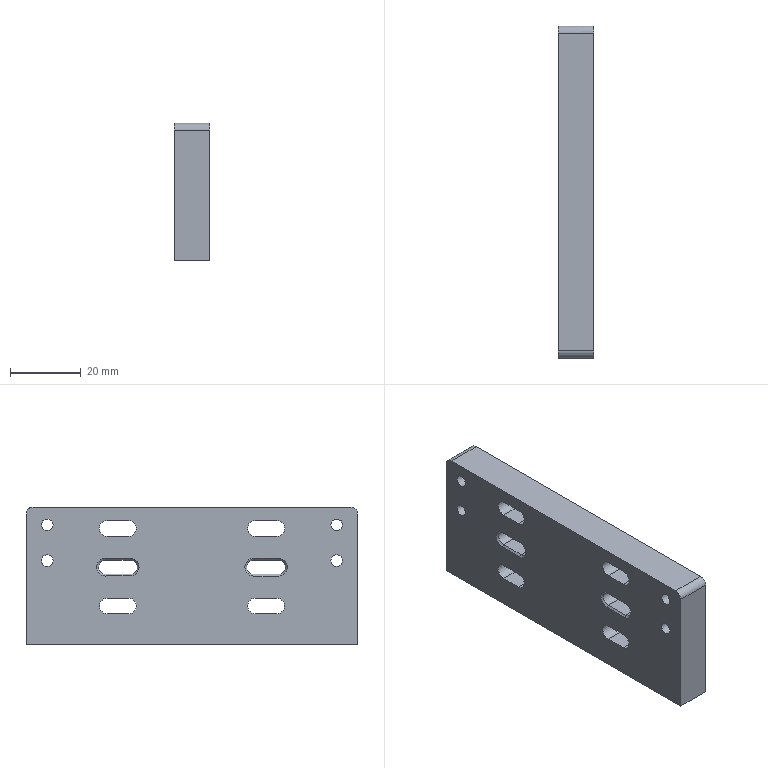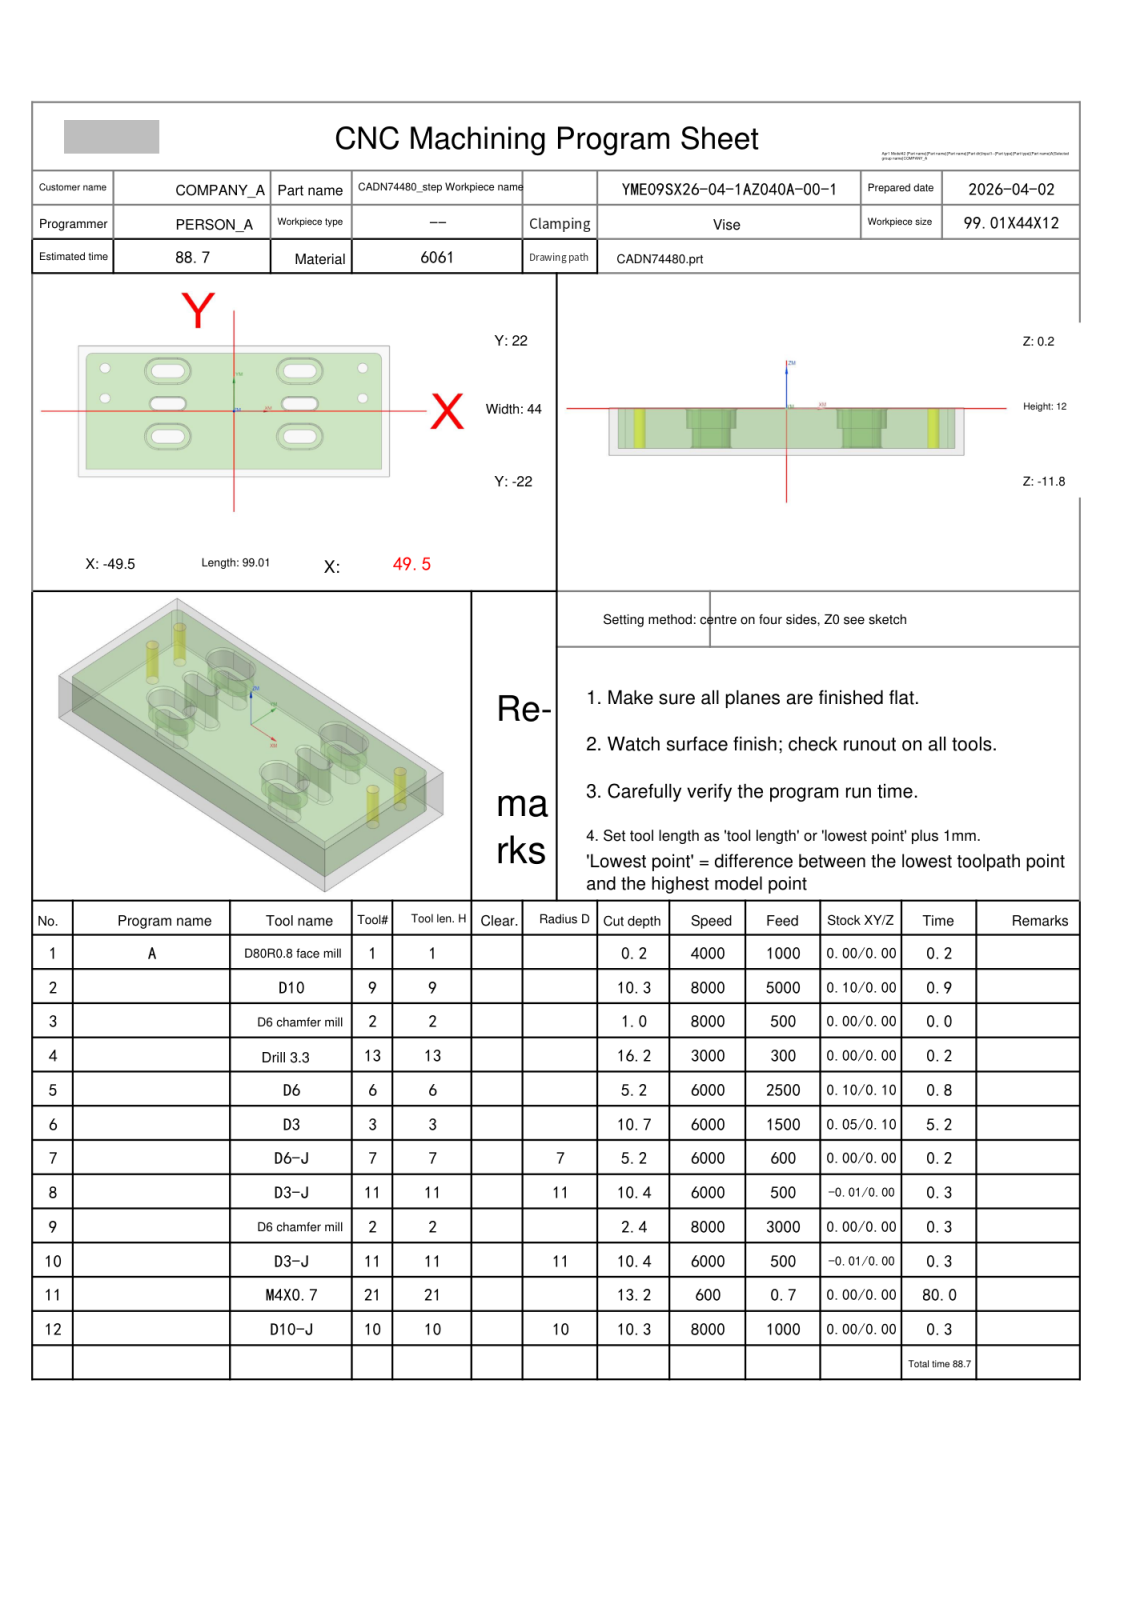NC program | NX | posted by the shop | part box 10.067 x 94 x 39 mm
Lines 1 to 937 of 4590:
%
O0001
(Machine time: 165.52 MIN)
(===Total Tool:10===)
(T1=D80R0.8 face mill D=80.  R=0.8  D-  H01 Z=0.    )
(T9=D10     D=10.  R=0.   D-  H09 Z=-10.1 )
(T2=D6 chamfer mill   D=6.   R=0.   D-  H02 Z=-2.2  )
(T13=Drill 3.3  D=3.3  DR_a=118 D-  H13 Z=-15.99)
(T6=D6      D=6.   R=0.   D-  H06 Z=-5.   )
(T3=D3      D=3.   R=0.   D-  H03 Z=-10.5 )
(T7=D6-J    D=6.   R=0.   D7  H07 Z=-5.   )
(T11=D3-J   D=3.   R=0.   D11 H11 Z=-10.2 )
(T21=M4X0.7 D=3.3  DR_a=180 D-  H21 Z=-13.  )
(T10=D10-J  D=10.  R=0.   D10 H10 Z=-10.1 )
G80 G90 G17 G49 G40
G91 G28 Z0
M01
N1 T01 M06
(D80R0.8 face mill  D=80. R=0.8 H=01 ce=0.00 di=0.00)
G00 G90 G54 X-92.004 Y0.0 M03 S4000
G43 H01 Z20.
M08
Z2.
G01 Z0.0 F1000.
X-87.004
X87.004
X92.004
Z2.
G00 Z20.
G91 G28 Z0.0
M05
M09
G91 G28 Z0.0
M01
N2 T09 M06
(D10  D=10. R=0. H=09 ce=0.10 di=0.00)
G00 G90 G54 X0.0 Y-24.6 M03 S8000
G43 H09 Z20.
M08
Z.5
G01 X-47.004 Z.38 F5000.
G02 X-52.104 Y-19.5 Z.359 I0.0 J5.1
G01 Y17.5 Z.265
G02 X-45.004 Y24.6 Z.236 I7.1 J0.0
G01 X45.004 Z.006
G02 X52.104 Y17.5 Z-.022 I0.0 J-7.1
G01 Y-19.5 Z-.117
G02 X47.004 Y-24.6 Z-.137 I-5.1 J0.0
G01 X-47.004 Z-.377
G02 X-52.104 Y-19.5 Z-.398 I0.0 J5.1
G01 Y17.5 Z-.492
G02 X-45.004 Y24.6 Z-.521 I7.1 J0.0
G01 X45.004 Z-.751
G02 X52.104 Y17.5 Z-.779 I0.0 J-7.1
G01 Y-19.5 Z-.874
G02 X47.004 Y-24.6 Z-.894 I-5.1 J0.0
G01 X-47.004 Z-1.134
G02 X-52.104 Y-19.5 Z-1.155 I0.0 J5.1
G01 Y17.5 Z-1.249
G02 X-45.004 Y24.6 Z-1.278 I7.1 J0.0
G01 X45.004 Z-1.508
G02 X52.104 Y17.5 Z-1.536 I0.0 J-7.1
G01 Y-19.5 Z-1.631
G02 X47.004 Y-24.6 Z-1.651 I-5.1 J0.0
G01 X-47.004 Z-1.892
G02 X-52.104 Y-19.5 Z-1.912 I0.0 J5.1
G01 Y17.5 Z-2.007
G02 X-45.004 Y24.6 Z-2.035 I7.1 J0.0
G01 X45.004 Z-2.265
G02 X52.104 Y17.5 Z-2.293 I0.0 J-7.1
G01 Y-19.5 Z-2.388
G02 X47.004 Y-24.6 Z-2.408 I-5.1 J0.0
G01 X-47.004 Z-2.649
G02 X-52.104 Y-19.5 Z-2.669 I0.0 J5.1
G01 Y17.5 Z-2.764
G02 X-45.004 Y24.6 Z-2.792 I7.1 J0.0
G01 X45.004 Z-3.022
G02 X52.104 Y17.5 Z-3.051 I0.0 J-7.1
G01 Y-19.5 Z-3.145
G02 X47.004 Y-24.6 Z-3.166 I-5.1 J0.0
G01 X-47.004 Z-3.406
G02 X-52.104 Y-19.5 Z-3.426 I0.0 J5.1
G01 Y17.5 Z-3.521
G02 X-45.004 Y24.6 Z-3.549 I7.1 J0.0
G01 X45.004 Z-3.779
G02 X52.104 Y17.5 Z-3.808 I0.0 J-7.1
G01 Y-19.5 Z-3.902
G02 X47.004 Y-24.6 Z-3.923 I-5.1 J0.0
G01 X-47.004 Z-4.163
G02 X-52.104 Y-19.5 Z-4.183 I0.0 J5.1
G01 Y17.5 Z-4.278
G02 X-45.004 Y24.6 Z-4.306 I7.1 J0.0
G01 X45.004 Z-4.536
G02 X52.104 Y17.5 Z-4.565 I0.0 J-7.1
G01 Y-19.5 Z-4.659
G02 X47.004 Y-24.6 Z-4.68 I-5.1 J0.0
G01 X-47.004 Z-4.92
G02 X-52.104 Y-19.5 Z-4.941 I0.0 J5.1
G01 Y17.5 Z-5.035
G02 X-45.004 Y24.6 Z-5.064 I7.1 J0.0
G01 X45.004 Z-5.294
G02 X52.104 Y17.5 Z-5.322 I0.0 J-7.1
G01 Y-19.5 Z-5.417
G02 X47.004 Y-24.6 Z-5.437 I-5.1 J0.0
G01 X-47.004 Z-5.677
G02 X-52.104 Y-19.5 Z-5.698 I0.0 J5.1
G01 Y17.5 Z-5.792
G02 X-45.004 Y24.6 Z-5.821 I7.1 J0.0
G01 X45.004 Z-6.051
G02 X52.104 Y17.5 Z-6.079 I0.0 J-7.1
G01 Y-19.5 Z-6.174
G02 X47.004 Y-24.6 Z-6.194 I-5.1 J0.0
G01 X-47.004 Z-6.434
G02 X-52.104 Y-19.5 Z-6.455 I0.0 J5.1
G01 Y17.5 Z-6.549
G02 X-45.004 Y24.6 Z-6.578 I7.1 J0.0
G01 X45.004 Z-6.808
G02 X52.104 Y17.5 Z-6.836 I0.0 J-7.1
G01 Y-19.5 Z-6.931
G02 X47.004 Y-24.6 Z-6.951 I-5.1 J0.0
G01 X-47.004 Z-7.192
G02 X-52.104 Y-19.5 Z-7.212 I0.0 J5.1
G01 Y17.5 Z-7.307
G02 X-45.004 Y24.6 Z-7.335 I7.1 J0.0
G01 X45.004 Z-7.565
G02 X52.104 Y17.5 Z-7.593 I0.0 J-7.1
G01 Y-19.5 Z-7.688
G02 X47.004 Y-24.6 Z-7.708 I-5.1 J0.0
G01 X-47.004 Z-7.949
G02 X-52.104 Y-19.5 Z-7.969 I0.0 J5.1
G01 Y17.5 Z-8.064
G02 X-45.004 Y24.6 Z-8.092 I7.1 J0.0
G01 X45.004 Z-8.322
G02 X52.104 Y17.5 Z-8.351 I0.0 J-7.1
G01 Y-19.5 Z-8.445
G02 X47.004 Y-24.6 Z-8.466 I-5.1 J0.0
G01 X-47.004 Z-8.706
G02 X-52.104 Y-19.5 Z-8.726 I0.0 J5.1
G01 Y17.5 Z-8.821
G02 X-45.004 Y24.6 Z-8.849 I7.1 J0.0
G01 X45.004 Z-9.079
G02 X52.104 Y17.5 Z-9.108 I0.0 J-7.1
G01 Y-19.5 Z-9.202
G02 X47.004 Y-24.6 Z-9.223 I-5.1 J0.0
G01 X-47.004 Z-9.463
G02 X-52.104 Y-19.5 Z-9.483 I0.0 J5.1
G01 Y17.5 Z-9.578
G02 X-45.004 Y24.6 Z-9.606 I7.1 J0.0
G01 X45.004 Z-9.836
G02 X52.104 Y17.5 Z-9.865 I0.0 J-7.1
G01 Y-19.5 Z-9.959
G02 X47.004 Y-24.6 Z-9.98 I-5.1 J0.0
G01 X0.0 Z-10.1
X-47.004
G02 X-52.104 Y-19.5 I0.0 J5.1
G01 Y17.5
G02 X-45.004 Y24.6 I7.1 J0.0
G01 X45.004
G02 X52.104 Y17.5 I0.0 J-7.1
G01 Y-19.5
G02 X47.004 Y-24.6 I-5.1 J0.0
G01 X0.0
X-.5
Z-9.1
G00 Z20.
G91 G28 Z0.0
M05
M09
G91 G28 Z0.0
M01
N3 T02 M06
(D6 chamfer mill  D=6. R=0. H=02 ce=0.00 di=0.00)
G00 G90 G54 X41.004 Y4.35 M03 S8000
G43 H02 Z20.
M08
G98 G81 X41.004 Y4.35 Z-.8 R1. F500.
Y14.5
X-40.996
Y4.35
G80
G00 Z20.
G91 G28 Z0.0
M05
M09
G91 G28 Z0.0
M01
N4 T13 M06
(Drill 3.3 D=3.3 DR_a=118 H=13)
G00 G90 G54 X41.004 Y4.35 M03 S3000
G43 H13 Z20.
M08
G98 G83 X41.004 Y4.35 Z-15.991 R1. F300. Q2.
Y14.5
X-40.996
Y4.35
G80
G00 Z20.
G91 G28 Z0.0
M05
M09
G91 G28 Z0.0
M01
N5 T06 M06
(D6  D=6. R=0. H=06 ce=0.10 di=0.10)
G00 G90 G54 X-20.996 Y14.4 M03 S6000
G43 H06 Z20.
M08
Z.5
G01 X-23.996 Z.467 F2500.
G03 X-24.896 Y13.5 Z.451 I0.0 J-.9
X-23.996 Y12.6 Z.435 I.9 J0.0
G01 X-17.996 Z.368
G03 X-17.096 Y13.5 Z.353 I0.0 J.9
X-17.996 Y14.4 Z.337 I-.9 J0.0
G01 X-23.996 Z.27
G03 X-24.896 Y13.5 Z.254 I0.0 J-.9
X-23.996 Y12.6 Z.239 I.9 J0.0
G01 X-17.996 Z.172
G03 X-17.096 Y13.5 Z.156 I0.0 J.9
X-17.996 Y14.4 Z.141 I-.9 J0.0
G01 X-23.996 Z.074
G03 X-24.896 Y13.5 Z.058 I0.0 J-.9
X-23.996 Y12.6 Z.042 I.9 J0.0
G01 X-17.996 Z-.024
G03 X-17.096 Y13.5 Z-.04 I0.0 J.9
X-17.996 Y14.4 Z-.056 I-.9 J0.0
G01 X-23.996 Z-.123
G03 X-24.896 Y13.5 Z-.138 I0.0 J-.9
X-23.996 Y12.6 Z-.154 I.9 J0.0
G01 X-17.996 Z-.221
G03 X-17.096 Y13.5 Z-.237 I0.0 J.9
X-17.996 Y14.4 Z-.252 I-.9 J0.0
G01 X-23.996 Z-.319
G03 X-24.896 Y13.5 Z-.335 I0.0 J-.9
X-23.996 Y12.6 Z-.351 I.9 J0.0
G01 X-17.996 Z-.417
G03 X-17.096 Y13.5 Z-.433 I0.0 J.9
X-17.996 Y14.4 Z-.449 I-.9 J0.0
G01 X-23.996 Z-.516
G03 X-24.896 Y13.5 Z-.531 I0.0 J-.9
X-23.996 Y12.6 Z-.547 I.9 J0.0
G01 X-17.996 Z-.614
G03 X-17.096 Y13.5 Z-.629 I0.0 J.9
X-17.996 Y14.4 Z-.645 I-.9 J0.0
G01 X-23.996 Z-.712
G03 X-24.896 Y13.5 Z-.728 I0.0 J-.9
X-23.996 Y12.6 Z-.743 I.9 J0.0
G01 X-17.996 Z-.81
G03 X-17.096 Y13.5 Z-.826 I0.0 J.9
X-17.996 Y14.4 Z-.842 I-.9 J0.0
G01 X-23.996 Z-.908
G03 X-24.896 Y13.5 Z-.924 I0.0 J-.9
X-23.996 Y12.6 Z-.94 I.9 J0.0
G01 X-17.996 Z-1.007
G03 X-17.096 Y13.5 Z-1.022 I0.0 J.9
X-17.996 Y14.4 Z-1.038 I-.9 J0.0
G01 X-23.996 Z-1.105
G03 X-24.896 Y13.5 Z-1.121 I0.0 J-.9
X-23.996 Y12.6 Z-1.136 I.9 J0.0
G01 X-17.996 Z-1.203
G03 X-17.096 Y13.5 Z-1.219 I0.0 J.9
X-17.996 Y14.4 Z-1.234 I-.9 J0.0
G01 X-23.996 Z-1.301
G03 X-24.896 Y13.5 Z-1.317 I0.0 J-.9
X-23.996 Y12.6 Z-1.333 I.9 J0.0
G01 X-17.996 Z-1.399
G03 X-17.096 Y13.5 Z-1.415 I0.0 J.9
X-17.996 Y14.4 Z-1.431 I-.9 J0.0
G01 X-23.996 Z-1.498
G03 X-24.896 Y13.5 Z-1.513 I0.0 J-.9
X-23.996 Y12.6 Z-1.529 I.9 J0.0
G01 X-17.996 Z-1.596
G03 X-17.096 Y13.5 Z-1.612 I0.0 J.9
X-17.996 Y14.4 Z-1.627 I-.9 J0.0
G01 X-23.996 Z-1.694
G03 X-24.896 Y13.5 Z-1.71 I0.0 J-.9
X-23.996 Y12.6 Z-1.726 I.9 J0.0
G01 X-17.996 Z-1.792
G03 X-17.096 Y13.5 Z-1.808 I0.0 J.9
X-17.996 Y14.4 Z-1.824 I-.9 J0.0
G01 X-23.996 Z-1.891
G03 X-24.896 Y13.5 Z-1.906 I0.0 J-.9
X-23.996 Y12.6 Z-1.922 I.9 J0.0
G01 X-17.996 Z-1.989
G03 X-17.096 Y13.5 Z-2.004 I0.0 J.9
X-17.996 Y14.4 Z-2.02 I-.9 J0.0
G01 X-23.996 Z-2.087
G03 X-24.896 Y13.5 Z-2.103 I0.0 J-.9
X-23.996 Y12.6 Z-2.118 I.9 J0.0
G01 X-17.996 Z-2.185
G03 X-17.096 Y13.5 Z-2.201 I0.0 J.9
X-17.996 Y14.4 Z-2.217 I-.9 J0.0
G01 X-23.996 Z-2.283
G03 X-24.896 Y13.5 Z-2.299 I0.0 J-.9
X-23.996 Y12.6 Z-2.315 I.9 J0.0
G01 X-17.996 Z-2.382
G03 X-17.096 Y13.5 Z-2.397 I0.0 J.9
X-17.996 Y14.4 Z-2.413 I-.9 J0.0
G01 X-23.996 Z-2.48
G03 X-24.896 Y13.5 Z-2.496 I0.0 J-.9
X-23.996 Y12.6 Z-2.511 I.9 J0.0
G01 X-17.996 Z-2.578
G03 X-17.096 Y13.5 Z-2.594 I0.0 J.9
X-17.996 Y14.4 Z-2.609 I-.9 J0.0
G01 X-23.996 Z-2.676
G03 X-24.896 Y13.5 Z-2.692 I0.0 J-.9
X-23.996 Y12.6 Z-2.708 I.9 J0.0
G01 X-17.996 Z-2.774
G03 X-17.096 Y13.5 Z-2.79 I0.0 J.9
X-17.996 Y14.4 Z-2.806 I-.9 J0.0
G01 X-23.996 Z-2.873
G03 X-24.896 Y13.5 Z-2.888 I0.0 J-.9
X-23.996 Y12.6 Z-2.904 I.9 J0.0
G01 X-17.996 Z-2.971
G03 X-17.096 Y13.5 Z-2.987 I0.0 J.9
X-17.996 Y14.4 Z-3.002 I-.9 J0.0
G01 X-23.996 Z-3.069
G03 X-24.896 Y13.5 Z-3.085 I0.0 J-.9
X-23.996 Y12.6 Z-3.101 I.9 J0.0
G01 X-17.996 Z-3.167
G03 X-17.096 Y13.5 Z-3.183 I0.0 J.9
X-17.996 Y14.4 Z-3.199 I-.9 J0.0
G01 X-23.996 Z-3.266
G03 X-24.896 Y13.5 Z-3.281 I0.0 J-.9
X-23.996 Y12.6 Z-3.297 I.9 J0.0
G01 X-17.996 Z-3.364
G03 X-17.096 Y13.5 Z-3.379 I0.0 J.9
X-17.996 Y14.4 Z-3.395 I-.9 J0.0
G01 X-23.996 Z-3.462
G03 X-24.896 Y13.5 Z-3.478 I0.0 J-.9
X-23.996 Y12.6 Z-3.493 I.9 J0.0
G01 X-17.996 Z-3.56
G03 X-17.096 Y13.5 Z-3.576 I0.0 J.9
X-17.996 Y14.4 Z-3.592 I-.9 J0.0
G01 X-23.996 Z-3.658
G03 X-24.896 Y13.5 Z-3.674 I0.0 J-.9
X-23.996 Y12.6 Z-3.69 I.9 J0.0
G01 X-17.996 Z-3.757
G03 X-17.096 Y13.5 Z-3.772 I0.0 J.9
X-17.996 Y14.4 Z-3.788 I-.9 J0.0
G01 X-23.996 Z-3.855
G03 X-24.896 Y13.5 Z-3.871 I0.0 J-.9
X-23.996 Y12.6 Z-3.886 I.9 J0.0
G01 X-17.996 Z-3.953
G03 X-17.096 Y13.5 Z-3.969 I0.0 J.9
X-17.996 Y14.4 Z-3.984 I-.9 J0.0
G01 X-23.996 Z-4.051
G03 X-24.896 Y13.5 Z-4.067 I0.0 J-.9
X-23.996 Y12.6 Z-4.083 I.9 J0.0
G01 X-17.996 Z-4.149
G03 X-17.096 Y13.5 Z-4.165 I0.0 J.9
X-17.996 Y14.4 Z-4.181 I-.9 J0.0
G01 X-23.996 Z-4.248
G03 X-24.896 Y13.5 Z-4.263 I0.0 J-.9
X-23.996 Y12.6 Z-4.279 I.9 J0.0
G01 X-17.996 Z-4.346
G03 X-17.096 Y13.5 Z-4.362 I0.0 J.9
X-17.996 Y14.4 Z-4.377 I-.9 J0.0
G01 X-23.996 Z-4.444
G03 X-24.896 Y13.5 Z-4.46 I0.0 J-.9
X-23.996 Y12.6 Z-4.476 I.9 J0.0
G01 X-17.996 Z-4.542
G03 X-17.096 Y13.5 Z-4.558 I0.0 J.9
X-17.996 Y14.4 Z-4.574 I-.9 J0.0
G01 X-23.996 Z-4.641
G03 X-24.896 Y13.5 Z-4.656 I0.0 J-.9
X-23.996 Y12.6 Z-4.672 I.9 J0.0
G01 X-17.996 Z-4.739
G03 X-17.096 Y13.5 Z-4.754 I0.0 J.9
X-17.996 Y14.4 Z-4.77 I-.9 J0.0
G01 X-23.996 Z-4.837
G03 X-24.896 Y13.5 Z-4.853 I0.0 J-.9
X-23.996 Y12.6 Z-4.868 I.9 J0.0
G01 X-17.996 Z-4.935
G03 X-17.096 Y13.5 Z-4.951 I0.0 J.9
X-17.996 Y14.4 Z-4.967 I-.9 J0.0
G01 X-20.996 Z-5.
X-23.996
G03 X-24.896 Y13.5 I0.0 J-.9
X-23.996 Y12.6 I.9 J0.0
G01 X-17.996
G03 X-17.096 Y13.5 I0.0 J.9
X-17.996 Y14.4 I-.9 J0.0
G01 X-20.996
X-21.496
Z-4.
G00 Z20.
X-20.996 Y-9.4
Z.5
G01 X-17.996 Z.467
G03 X-17.096 Y-8.5 Z.451 I0.0 J.9
X-17.996 Y-7.6 Z.435 I-.9 J0.0
G01 X-23.996 Z.368
G03 X-24.896 Y-8.5 Z.353 I0.0 J-.9
X-23.996 Y-9.4 Z.337 I.9 J0.0
G01 X-17.996 Z.27
G03 X-17.096 Y-8.5 Z.254 I0.0 J.9
X-17.996 Y-7.6 Z.239 I-.9 J0.0
G01 X-23.996 Z.172
G03 X-24.896 Y-8.5 Z.156 I0.0 J-.9
X-23.996 Y-9.4 Z.141 I.9 J0.0
G01 X-17.996 Z.074
G03 X-17.096 Y-8.5 Z.058 I0.0 J.9
X-17.996 Y-7.6 Z.042 I-.9 J0.0
G01 X-23.996 Z-.024
G03 X-24.896 Y-8.5 Z-.04 I0.0 J-.9
X-23.996 Y-9.4 Z-.056 I.9 J0.0
G01 X-17.996 Z-.123
G03 X-17.096 Y-8.5 Z-.138 I0.0 J.9
X-17.996 Y-7.6 Z-.154 I-.9 J0.0
G01 X-23.996 Z-.221
G03 X-24.896 Y-8.5 Z-.237 I0.0 J-.9
X-23.996 Y-9.4 Z-.252 I.9 J0.0
G01 X-17.996 Z-.319
G03 X-17.096 Y-8.5 Z-.335 I0.0 J.9
X-17.996 Y-7.6 Z-.351 I-.9 J0.0
G01 X-23.996 Z-.417
G03 X-24.896 Y-8.5 Z-.433 I0.0 J-.9
X-23.996 Y-9.4 Z-.449 I.9 J0.0
G01 X-17.996 Z-.516
G03 X-17.096 Y-8.5 Z-.531 I0.0 J.9
X-17.996 Y-7.6 Z-.547 I-.9 J0.0
G01 X-23.996 Z-.614
G03 X-24.896 Y-8.5 Z-.629 I0.0 J-.9
X-23.996 Y-9.4 Z-.645 I.9 J0.0
G01 X-17.996 Z-.712
G03 X-17.096 Y-8.5 Z-.728 I0.0 J.9
X-17.996 Y-7.6 Z-.743 I-.9 J0.0
G01 X-23.996 Z-.81
G03 X-24.896 Y-8.5 Z-.826 I0.0 J-.9
X-23.996 Y-9.4 Z-.842 I.9 J0.0
G01 X-17.996 Z-.908
G03 X-17.096 Y-8.5 Z-.924 I0.0 J.9
X-17.996 Y-7.6 Z-.94 I-.9 J0.0
G01 X-23.996 Z-1.007
G03 X-24.896 Y-8.5 Z-1.022 I0.0 J-.9
X-23.996 Y-9.4 Z-1.038 I.9 J0.0
G01 X-17.996 Z-1.105
G03 X-17.096 Y-8.5 Z-1.121 I0.0 J.9
X-17.996 Y-7.6 Z-1.136 I-.9 J0.0
G01 X-23.996 Z-1.203
G03 X-24.896 Y-8.5 Z-1.219 I0.0 J-.9
X-23.996 Y-9.4 Z-1.234 I.9 J0.0
G01 X-17.996 Z-1.301
G03 X-17.096 Y-8.5 Z-1.317 I0.0 J.9
X-17.996 Y-7.6 Z-1.333 I-.9 J0.0
G01 X-23.996 Z-1.399
G03 X-24.896 Y-8.5 Z-1.415 I0.0 J-.9
X-23.996 Y-9.4 Z-1.431 I.9 J0.0
G01 X-17.996 Z-1.498
G03 X-17.096 Y-8.5 Z-1.513 I0.0 J.9
X-17.996 Y-7.6 Z-1.529 I-.9 J0.0
G01 X-23.996 Z-1.596
G03 X-24.896 Y-8.5 Z-1.612 I0.0 J-.9
X-23.996 Y-9.4 Z-1.627 I.9 J0.0
G01 X-17.996 Z-1.694
G03 X-17.096 Y-8.5 Z-1.71 I0.0 J.9
X-17.996 Y-7.6 Z-1.726 I-.9 J0.0
G01 X-23.996 Z-1.792
G03 X-24.896 Y-8.5 Z-1.808 I0.0 J-.9
X-23.996 Y-9.4 Z-1.824 I.9 J0.0
G01 X-17.996 Z-1.891
G03 X-17.096 Y-8.5 Z-1.906 I0.0 J.9
X-17.996 Y-7.6 Z-1.922 I-.9 J0.0
G01 X-23.996 Z-1.989
G03 X-24.896 Y-8.5 Z-2.004 I0.0 J-.9
X-23.996 Y-9.4 Z-2.02 I.9 J0.0
G01 X-17.996 Z-2.087
G03 X-17.096 Y-8.5 Z-2.103 I0.0 J.9
X-17.996 Y-7.6 Z-2.118 I-.9 J0.0
G01 X-23.996 Z-2.185
G03 X-24.896 Y-8.5 Z-2.201 I0.0 J-.9
X-23.996 Y-9.4 Z-2.217 I.9 J0.0
G01 X-17.996 Z-2.283
G03 X-17.096 Y-8.5 Z-2.299 I0.0 J.9
X-17.996 Y-7.6 Z-2.315 I-.9 J0.0
G01 X-23.996 Z-2.382
G03 X-24.896 Y-8.5 Z-2.397 I0.0 J-.9
X-23.996 Y-9.4 Z-2.413 I.9 J0.0
G01 X-17.996 Z-2.48
G03 X-17.096 Y-8.5 Z-2.496 I0.0 J.9
X-17.996 Y-7.6 Z-2.511 I-.9 J0.0
G01 X-23.996 Z-2.578
G03 X-24.896 Y-8.5 Z-2.594 I0.0 J-.9
X-23.996 Y-9.4 Z-2.609 I.9 J0.0
G01 X-17.996 Z-2.676
G03 X-17.096 Y-8.5 Z-2.692 I0.0 J.9
X-17.996 Y-7.6 Z-2.708 I-.9 J0.0
G01 X-23.996 Z-2.774
G03 X-24.896 Y-8.5 Z-2.79 I0.0 J-.9
X-23.996 Y-9.4 Z-2.806 I.9 J0.0
G01 X-17.996 Z-2.873
G03 X-17.096 Y-8.5 Z-2.888 I0.0 J.9
X-17.996 Y-7.6 Z-2.904 I-.9 J0.0
G01 X-23.996 Z-2.971
G03 X-24.896 Y-8.5 Z-2.987 I0.0 J-.9
X-23.996 Y-9.4 Z-3.002 I.9 J0.0
G01 X-17.996 Z-3.069
G03 X-17.096 Y-8.5 Z-3.085 I0.0 J.9
X-17.996 Y-7.6 Z-3.101 I-.9 J0.0
G01 X-23.996 Z-3.167
G03 X-24.896 Y-8.5 Z-3.183 I0.0 J-.9
X-23.996 Y-9.4 Z-3.199 I.9 J0.0
G01 X-17.996 Z-3.266
G03 X-17.096 Y-8.5 Z-3.281 I0.0 J.9
X-17.996 Y-7.6 Z-3.297 I-.9 J0.0
G01 X-23.996 Z-3.364
G03 X-24.896 Y-8.5 Z-3.379 I0.0 J-.9
X-23.996 Y-9.4 Z-3.395 I.9 J0.0
G01 X-17.996 Z-3.462
G03 X-17.096 Y-8.5 Z-3.478 I0.0 J.9
X-17.996 Y-7.6 Z-3.493 I-.9 J0.0
G01 X-23.996 Z-3.56
G03 X-24.896 Y-8.5 Z-3.576 I0.0 J-.9
X-23.996 Y-9.4 Z-3.592 I.9 J0.0
G01 X-17.996 Z-3.658
G03 X-17.096 Y-8.5 Z-3.674 I0.0 J.9
X-17.996 Y-7.6 Z-3.69 I-.9 J0.0
G01 X-23.996 Z-3.757
G03 X-24.896 Y-8.5 Z-3.772 I0.0 J-.9
X-23.996 Y-9.4 Z-3.788 I.9 J0.0
G01 X-17.996 Z-3.855
G03 X-17.096 Y-8.5 Z-3.871 I0.0 J.9
X-17.996 Y-7.6 Z-3.886 I-.9 J0.0
G01 X-23.996 Z-3.953
G03 X-24.896 Y-8.5 Z-3.969 I0.0 J-.9
X-23.996 Y-9.4 Z-3.984 I.9 J0.0
G01 X-17.996 Z-4.051
G03 X-17.096 Y-8.5 Z-4.067 I0.0 J.9
X-17.996 Y-7.6 Z-4.083 I-.9 J0.0
G01 X-23.996 Z-4.149
G03 X-24.896 Y-8.5 Z-4.165 I0.0 J-.9
X-23.996 Y-9.4 Z-4.181 I.9 J0.0
G01 X-17.996 Z-4.248
G03 X-17.096 Y-8.5 Z-4.263 I0.0 J.9
X-17.996 Y-7.6 Z-4.279 I-.9 J0.0
G01 X-23.996 Z-4.346
G03 X-24.896 Y-8.5 Z-4.362 I0.0 J-.9
X-23.996 Y-9.4 Z-4.377 I.9 J0.0
G01 X-17.996 Z-4.444
G03 X-17.096 Y-8.5 Z-4.46 I0.0 J.9
X-17.996 Y-7.6 Z-4.476 I-.9 J0.0
G01 X-23.996 Z-4.542
G03 X-24.896 Y-8.5 Z-4.558 I0.0 J-.9
X-23.996 Y-9.4 Z-4.574 I.9 J0.0
G01 X-17.996 Z-4.641
G03 X-17.096 Y-8.5 Z-4.656 I0.0 J.9
X-17.996 Y-7.6 Z-4.672 I-.9 J0.0
G01 X-23.996 Z-4.739
G03 X-24.896 Y-8.5 Z-4.754 I0.0 J-.9
X-23.996 Y-9.4 Z-4.77 I.9 J0.0
G01 X-17.996 Z-4.837
G03 X-17.096 Y-8.5 Z-4.853 I0.0 J.9
X-17.996 Y-7.6 Z-4.868 I-.9 J0.0
G01 X-23.996 Z-4.935
G03 X-24.896 Y-8.5 Z-4.951 I0.0 J-.9
X-23.996 Y-9.4 Z-4.967 I.9 J0.0
G01 X-20.996 Z-5.
X-17.996
G03 X-17.096 Y-8.5 I0.0 J.9
X-17.996 Y-7.6 I-.9 J0.0
G01 X-23.996
G03 X-24.896 Y-8.5 I0.0 J-.9
X-23.996 Y-9.4 I.9 J0.0
G01 X-20.996
X-20.496
Z-4.
G00 Z20.
X21.004
Z.5
G01 X24.004 Z.467
G03 X24.904 Y-8.5 Z.451 I0.0 J.9
X24.004 Y-7.6 Z.435 I-.9 J0.0
G01 X18.004 Z.368
G03 X17.104 Y-8.5 Z.353 I0.0 J-.9
X18.004 Y-9.4 Z.337 I.9 J0.0
G01 X24.004 Z.27
G03 X24.904 Y-8.5 Z.254 I0.0 J.9
X24.004 Y-7.6 Z.239 I-.9 J0.0
G01 X18.004 Z.172
G03 X17.104 Y-8.5 Z.156 I0.0 J-.9
X18.004 Y-9.4 Z.141 I.9 J0.0
G01 X24.004 Z.074
G03 X24.904 Y-8.5 Z.058 I0.0 J.9
X24.004 Y-7.6 Z.042 I-.9 J0.0
G01 X18.004 Z-.024
G03 X17.104 Y-8.5 Z-.04 I0.0 J-.9
X18.004 Y-9.4 Z-.056 I.9 J0.0
G01 X24.004 Z-.123
G03 X24.904 Y-8.5 Z-.138 I0.0 J.9
X24.004 Y-7.6 Z-.154 I-.9 J0.0
G01 X18.004 Z-.221
G03 X17.104 Y-8.5 Z-.237 I0.0 J-.9
X18.004 Y-9.4 Z-.252 I.9 J0.0
G01 X24.004 Z-.319
G03 X24.904 Y-8.5 Z-.335 I0.0 J.9
X24.004 Y-7.6 Z-.351 I-.9 J0.0
G01 X18.004 Z-.417
G03 X17.104 Y-8.5 Z-.433 I0.0 J-.9
X18.004 Y-9.4 Z-.449 I.9 J0.0
G01 X24.004 Z-.516
G03 X24.904 Y-8.5 Z-.531 I0.0 J.9
X24.004 Y-7.6 Z-.547 I-.9 J0.0
G01 X18.004 Z-.614
G03 X17.104 Y-8.5 Z-.629 I0.0 J-.9
X18.004 Y-9.4 Z-.645 I.9 J0.0
G01 X24.004 Z-.712
G03 X24.904 Y-8.5 Z-.728 I0.0 J.9
X24.004 Y-7.6 Z-.743 I-.9 J0.0
G01 X18.004 Z-.81
G03 X17.104 Y-8.5 Z-.826 I0.0 J-.9
X18.004 Y-9.4 Z-.842 I.9 J0.0
G01 X24.004 Z-.908
G03 X24.904 Y-8.5 Z-.924 I0.0 J.9
X24.004 Y-7.6 Z-.94 I-.9 J0.0
G01 X18.004 Z-1.007
G03 X17.104 Y-8.5 Z-1.022 I0.0 J-.9
X18.004 Y-9.4 Z-1.038 I.9 J0.0
G01 X24.004 Z-1.105
G03 X24.904 Y-8.5 Z-1.121 I0.0 J.9
X24.004 Y-7.6 Z-1.136 I-.9 J0.0
G01 X18.004 Z-1.203
G03 X17.104 Y-8.5 Z-1.219 I0.0 J-.9
X18.004 Y-9.4 Z-1.234 I.9 J0.0
G01 X24.004 Z-1.301
G03 X24.904 Y-8.5 Z-1.317 I0.0 J.9
X24.004 Y-7.6 Z-1.333 I-.9 J0.0
G01 X18.004 Z-1.399
G03 X17.104 Y-8.5 Z-1.415 I0.0 J-.9
X18.004 Y-9.4 Z-1.431 I.9 J0.0
G01 X24.004 Z-1.498
G03 X24.904 Y-8.5 Z-1.513 I0.0 J.9
X24.004 Y-7.6 Z-1.529 I-.9 J0.0
G01 X18.004 Z-1.596
G03 X17.104 Y-8.5 Z-1.612 I0.0 J-.9
X18.004 Y-9.4 Z-1.627 I.9 J0.0
G01 X24.004 Z-1.694
G03 X24.904 Y-8.5 Z-1.71 I0.0 J.9
X24.004 Y-7.6 Z-1.726 I-.9 J0.0
G01 X18.004 Z-1.792
G03 X17.104 Y-8.5 Z-1.808 I0.0 J-.9
X18.004 Y-9.4 Z-1.824 I.9 J0.0
G01 X24.004 Z-1.891
G03 X24.904 Y-8.5 Z-1.906 I0.0 J.9
X24.004 Y-7.6 Z-1.922 I-.9 J0.0
G01 X18.004 Z-1.989
G03 X17.104 Y-8.5 Z-2.004 I0.0 J-.9
X18.004 Y-9.4 Z-2.02 I.9 J0.0
G01 X24.004 Z-2.087
G03 X24.904 Y-8.5 Z-2.103 I0.0 J.9
X24.004 Y-7.6 Z-2.118 I-.9 J0.0
G01 X18.004 Z-2.185
G03 X17.104 Y-8.5 Z-2.201 I0.0 J-.9
X18.004 Y-9.4 Z-2.217 I.9 J0.0
G01 X24.004 Z-2.283
G03 X24.904 Y-8.5 Z-2.299 I0.0 J.9
X24.004 Y-7.6 Z-2.315 I-.9 J0.0
G01 X18.004 Z-2.382
G03 X17.104 Y-8.5 Z-2.397 I0.0 J-.9
X18.004 Y-9.4 Z-2.413 I.9 J0.0
G01 X24.004 Z-2.48
G03 X24.904 Y-8.5 Z-2.496 I0.0 J.9
X24.004 Y-7.6 Z-2.511 I-.9 J0.0
G01 X18.004 Z-2.578
G03 X17.104 Y-8.5 Z-2.594 I0.0 J-.9
X18.004 Y-9.4 Z-2.609 I.9 J0.0
G01 X24.004 Z-2.676
G03 X24.904 Y-8.5 Z-2.692 I0.0 J.9
X24.004 Y-7.6 Z-2.708 I-.9 J0.0
G01 X18.004 Z-2.774
G03 X17.104 Y-8.5 Z-2.79 I0.0 J-.9
X18.004 Y-9.4 Z-2.806 I.9 J0.0
G01 X24.004 Z-2.873
G03 X24.904 Y-8.5 Z-2.888 I0.0 J.9
X24.004 Y-7.6 Z-2.904 I-.9 J0.0
G01 X18.004 Z-2.971
G03 X17.104 Y-8.5 Z-2.987 I0.0 J-.9
X18.004 Y-9.4 Z-3.002 I.9 J0.0
G01 X24.004 Z-3.069
G03 X24.904 Y-8.5 Z-3.085 I0.0 J.9
X24.004 Y-7.6 Z-3.101 I-.9 J0.0
G01 X18.004 Z-3.167
G03 X17.104 Y-8.5 Z-3.183 I0.0 J-.9
X18.004 Y-9.4 Z-3.199 I.9 J0.0
G01 X24.004 Z-3.266
G03 X24.904 Y-8.5 Z-3.281 I0.0 J.9
X24.004 Y-7.6 Z-3.297 I-.9 J0.0
G01 X18.004 Z-3.364
G03 X17.104 Y-8.5 Z-3.379 I0.0 J-.9
X18.004 Y-9.4 Z-3.395 I.9 J0.0
G01 X24.004 Z-3.462
G03 X24.904 Y-8.5 Z-3.478 I0.0 J.9
X24.004 Y-7.6 Z-3.493 I-.9 J0.0
G01 X18.004 Z-3.56
G03 X17.104 Y-8.5 Z-3.576 I0.0 J-.9
X18.004 Y-9.4 Z-3.592 I.9 J0.0
G01 X24.004 Z-3.658
G03 X24.904 Y-8.5 Z-3.674 I0.0 J.9
X24.004 Y-7.6 Z-3.69 I-.9 J0.0
G01 X18.004 Z-3.757
G03 X17.104 Y-8.5 Z-3.772 I0.0 J-.9
X18.004 Y-9.4 Z-3.788 I.9 J0.0
G01 X24.004 Z-3.855
G03 X24.904 Y-8.5 Z-3.871 I0.0 J.9
X24.004 Y-7.6 Z-3.886 I-.9 J0.0
G01 X18.004 Z-3.953
G03 X17.104 Y-8.5 Z-3.969 I0.0 J-.9
X18.004 Y-9.4 Z-3.984 I.9 J0.0
G01 X24.004 Z-4.051
G03 X24.904 Y-8.5 Z-4.067 I0.0 J.9
X24.004 Y-7.6 Z-4.083 I-.9 J0.0
G01 X18.004 Z-4.149
G03 X17.104 Y-8.5 Z-4.165 I0.0 J-.9
X18.004 Y-9.4 Z-4.181 I.9 J0.0
G01 X24.004 Z-4.248
G03 X24.904 Y-8.5 Z-4.263 I0.0 J.9
X24.004 Y-7.6 Z-4.279 I-.9 J0.0
G01 X18.004 Z-4.346
G03 X17.104 Y-8.5 Z-4.362 I0.0 J-.9
X18.004 Y-9.4 Z-4.377 I.9 J0.0
G01 X24.004 Z-4.444
G03 X24.904 Y-8.5 Z-4.46 I0.0 J.9
X24.004 Y-7.6 Z-4.476 I-.9 J0.0
G01 X18.004 Z-4.542
G03 X17.104 Y-8.5 Z-4.558 I0.0 J-.9
X18.004 Y-9.4 Z-4.574 I.9 J0.0
G01 X24.004 Z-4.641
G03 X24.904 Y-8.5 Z-4.656 I0.0 J.9
X24.004 Y-7.6 Z-4.672 I-.9 J0.0
G01 X18.004 Z-4.739
G03 X17.104 Y-8.5 Z-4.754 I0.0 J-.9
X18.004 Y-9.4 Z-4.77 I.9 J0.0
G01 X24.004 Z-4.837
G03 X24.904 Y-8.5 Z-4.853 I0.0 J.9
X24.004 Y-7.6 Z-4.868 I-.9 J0.0
G01 X18.004 Z-4.935
G03 X17.104 Y-8.5 Z-4.951 I0.0 J-.9
X18.004 Y-9.4 Z-4.967 I.9 J0.0
G01 X21.004 Z-5.
X24.004
G03 X24.904 Y-8.5 I0.0 J.9
X24.004 Y-7.6 I-.9 J0.0
G01 X18.004
G03 X17.104 Y-8.5 I0.0 J-.9
X18.004 Y-9.4 I.9 J0.0
G01 X21.004
X21.504
Z-4.
G00 Z20.
X21.004 Y14.4
Z.5
G01 X18.004 Z.467
G03 X17.104 Y13.5 Z.451 I0.0 J-.9
X18.004 Y12.6 Z.435 I.9 J0.0
G01 X24.004 Z.368
G03 X24.904 Y13.5 Z.353 I0.0 J.9
X24.004 Y14.4 Z.337 I-.9 J0.0
G01 X18.004 Z.27
G03 X17.104 Y13.5 Z.254 I0.0 J-.9
X18.004 Y12.6 Z.239 I.9 J0.0
G01 X24.004 Z.172
G03 X24.904 Y13.5 Z.156 I0.0 J.9
X24.004 Y14.4 Z.141 I-.9 J0.0
G01 X18.004 Z.074
G03 X17.104 Y13.5 Z.058 I0.0 J-.9
X18.004 Y12.6 Z.042 I.9 J0.0
G01 X24.004 Z-.024
G03 X24.904 Y13.5 Z-.04 I0.0 J.9
X24.004 Y14.4 Z-.056 I-.9 J0.0
G01 X18.004 Z-.123
G03 X17.104 Y13.5 Z-.138 I0.0 J-.9
X18.004 Y12.6 Z-.154 I.9 J0.0
G01 X24.004 Z-.221
G03 X24.904 Y13.5 Z-.237 I0.0 J.9
X24.004 Y14.4 Z-.252 I-.9 J0.0
G01 X18.004 Z-.319
G03 X17.104 Y13.5 Z-.335 I0.0 J-.9
X18.004 Y12.6 Z-.351 I.9 J0.0
G01 X24.004 Z-.417
G03 X24.904 Y13.5 Z-.433 I0.0 J.9
X24.004 Y14.4 Z-.449 I-.9 J0.0
G01 X18.004 Z-.516
G03 X17.104 Y13.5 Z-.531 I0.0 J-.9
X18.004 Y12.6 Z-.547 I.9 J0.0
G01 X24.004 Z-.614
G03 X24.904 Y13.5 Z-.629 I0.0 J.9
X24.004 Y14.4 Z-.645 I-.9 J0.0
G01 X18.004 Z-.712
G03 X17.104 Y13.5 Z-.728 I0.0 J-.9
X18.004 Y12.6 Z-.743 I.9 J0.0
G01 X24.004 Z-.81
G03 X24.904 Y13.5 Z-.826 I0.0 J.9
X24.004 Y14.4 Z-.842 I-.9 J0.0
G01 X18.004 Z-.908
G03 X17.104 Y13.5 Z-.924 I0.0 J-.9
X18.004 Y12.6 Z-.94 I.9 J0.0
G01 X24.004 Z-1.007
G03 X24.904 Y13.5 Z-1.022 I0.0 J.9
X24.004 Y14.4 Z-1.038 I-.9 J0.0
G01 X18.004 Z-1.105
G03 X17.104 Y13.5 Z-1.121 I0.0 J-.9
X18.004 Y12.6 Z-1.136 I.9 J0.0
G01 X24.004 Z-1.203
G03 X24.904 Y13.5 Z-1.219 I0.0 J.9
X24.004 Y14.4 Z-1.234 I-.9 J0.0
G01 X18.004 Z-1.301
G03 X17.104 Y13.5 Z-1.317 I0.0 J-.9
X18.004 Y12.6 Z-1.333 I.9 J0.0
G01 X24.004 Z-1.399
G03 X24.904 Y13.5 Z-1.415 I0.0 J.9
X24.004 Y14.4 Z-1.431 I-.9 J0.0
G01 X18.004 Z-1.498
G03 X17.104 Y13.5 Z-1.513 I0.0 J-.9
X18.004 Y12.6 Z-1.529 I.9 J0.0
G01 X24.004 Z-1.596
G03 X24.904 Y13.5 Z-1.612 I0.0 J.9
X24.004 Y14.4 Z-1.627 I-.9 J0.0
G01 X18.004 Z-1.694
G03 X17.104 Y13.5 Z-1.71 I0.0 J-.9
X18.004 Y12.6 Z-1.726 I.9 J0.0
G01 X24.004 Z-1.792
G03 X24.904 Y13.5 Z-1.808 I0.0 J.9
X24.004 Y14.4 Z-1.824 I-.9 J0.0
G01 X18.004 Z-1.891
G03 X17.104 Y13.5 Z-1.906 I0.0 J-.9
X18.004 Y12.6 Z-1.922 I.9 J0.0
G01 X24.004 Z-1.989
G03 X24.904 Y13.5 Z-2.004 I0.0 J.9
X24.004 Y14.4 Z-2.02 I-.9 J0.0
G01 X18.004 Z-2.087
G03 X17.104 Y13.5 Z-2.103 I0.0 J-.9
X18.004 Y12.6 Z-2.118 I.9 J0.0
G01 X24.004 Z-2.185
G03 X24.904 Y13.5 Z-2.201 I0.0 J.9
X24.004 Y14.4 Z-2.217 I-.9 J0.0
G01 X18.004 Z-2.283
G03 X17.104 Y13.5 Z-2.299 I0.0 J-.9
X18.004 Y12.6 Z-2.315 I.9 J0.0
G01 X24.004 Z-2.382
G03 X24.904 Y13.5 Z-2.397 I0.0 J.9
X24.004 Y14.4 Z-2.413 I-.9 J0.0
G01 X18.004 Z-2.48
G03 X17.104 Y13.5 Z-2.496 I0.0 J-.9
X18.004 Y12.6 Z-2.511 I.9 J0.0
G01 X24.004 Z-2.578
G03 X24.904 Y13.5 Z-2.594 I0.0 J.9
X24.004 Y14.4 Z-2.609 I-.9 J0.0
G01 X18.004 Z-2.676
G03 X17.104 Y13.5 Z-2.692 I0.0 J-.9
X18.004 Y12.6 Z-2.708 I.9 J0.0
G01 X24.004 Z-2.774
G03 X24.904 Y13.5 Z-2.79 I0.0 J.9
X24.004 Y14.4 Z-2.806 I-.9 J0.0
G01 X18.004 Z-2.873
G03 X17.104 Y13.5 Z-2.888 I0.0 J-.9
X18.004 Y12.6 Z-2.904 I.9 J0.0
G01 X24.004 Z-2.971
G03 X24.904 Y13.5 Z-2.987 I0.0 J.9
X24.004 Y14.4 Z-3.002 I-.9 J0.0
G01 X18.004 Z-3.069
G03 X17.104 Y13.5 Z-3.085 I0.0 J-.9
X18.004 Y12.6 Z-3.101 I.9 J0.0
G01 X24.004 Z-3.167
G03 X24.904 Y13.5 Z-3.183 I0.0 J.9
X24.004 Y14.4 Z-3.199 I-.9 J0.0
G01 X18.004 Z-3.266
G03 X17.104 Y13.5 Z-3.281 I0.0 J-.9
X18.004 Y12.6 Z-3.297 I.9 J0.0
G01 X24.004 Z-3.364
G03 X24.904 Y13.5 Z-3.379 I0.0 J.9
X24.004 Y14.4 Z-3.395 I-.9 J0.0
G01 X18.004 Z-3.462
G03 X17.104 Y13.5 Z-3.478 I0.0 J-.9
X18.004 Y12.6 Z-3.493 I.9 J0.0
G01 X24.004 Z-3.56
G03 X24.904 Y13.5 Z-3.576 I0.0 J.9
X24.004 Y14.4 Z-3.592 I-.9 J0.0
G01 X18.004 Z-3.658
G03 X17.104 Y13.5 Z-3.674 I0.0 J-.9
X18.004 Y12.6 Z-3.69 I.9 J0.0
G01 X24.004 Z-3.757
G03 X24.904 Y13.5 Z-3.772 I0.0 J.9
X24.004 Y14.4 Z-3.788 I-.9 J0.0
G01 X18.004 Z-3.855
G03 X17.104 Y13.5 Z-3.871 I0.0 J-.9
X18.004 Y12.6 Z-3.886 I.9 J0.0
G01 X24.004 Z-3.953
G03 X24.904 Y13.5 Z-3.969 I0.0 J.9
X24.004 Y14.4 Z-3.984 I-.9 J0.0
G01 X18.004 Z-4.051
G03 X17.104 Y13.5 Z-4.067 I0.0 J-.9
X18.004 Y12.6 Z-4.083 I.9 J0.0
G01 X24.004 Z-4.149
G03 X24.904 Y13.5 Z-4.165 I0.0 J.9
X24.004 Y14.4 Z-4.181 I-.9 J0.0
G01 X18.004 Z-4.248
G03 X17.104 Y13.5 Z-4.263 I0.0 J-.9
X18.004 Y12.6 Z-4.279 I.9 J0.0
G01 X24.004 Z-4.346
G03 X24.904 Y13.5 Z-4.362 I0.0 J.9
X24.004 Y14.4 Z-4.377 I-.9 J0.0
G01 X18.004 Z-4.444
G03 X17.104 Y13.5 Z-4.46 I0.0 J-.9
X18.004 Y12.6 Z-4.476 I.9 J0.0
G01 X24.004 Z-4.542
G03 X24.904 Y13.5 Z-4.558 I0.0 J.9
X24.004 Y14.4 Z-4.574 I-.9 J0.0
G01 X18.004 Z-4.641
G03 X17.104 Y13.5 Z-4.656 I0.0 J-.9
X18.004 Y12.6 Z-4.672 I.9 J0.0
G01 X24.004 Z-4.739
G03 X24.904 Y13.5 Z-4.754 I0.0 J.9
X24.004 Y14.4 Z-4.77 I-.9 J0.0
G01 X18.004 Z-4.837
G03 X17.104 Y13.5 Z-4.853 I0.0 J-.9
X18.004 Y12.6 Z-4.868 I.9 J0.0
G01 X24.004 Z-4.935
G03 X24.904 Y13.5 Z-4.951 I0.0 J.9
X24.004 Y14.4 Z-4.967 I-.9 J0.0
G01 X21.004 Z-5.
X18.004
G03 X17.104 Y13.5 I0.0 J-.9
X18.004 Y12.6 I.9 J0.0
G01 X24.004
G03 X24.904 Y13.5 I0.0 J.9
X24.004 Y14.4 I-.9 J0.0
G01 X21.004
X20.504
Z-4.
G00 Z20.
G91 G28 Z0.0
M05
M09
G91 G28 Z0.0
M01